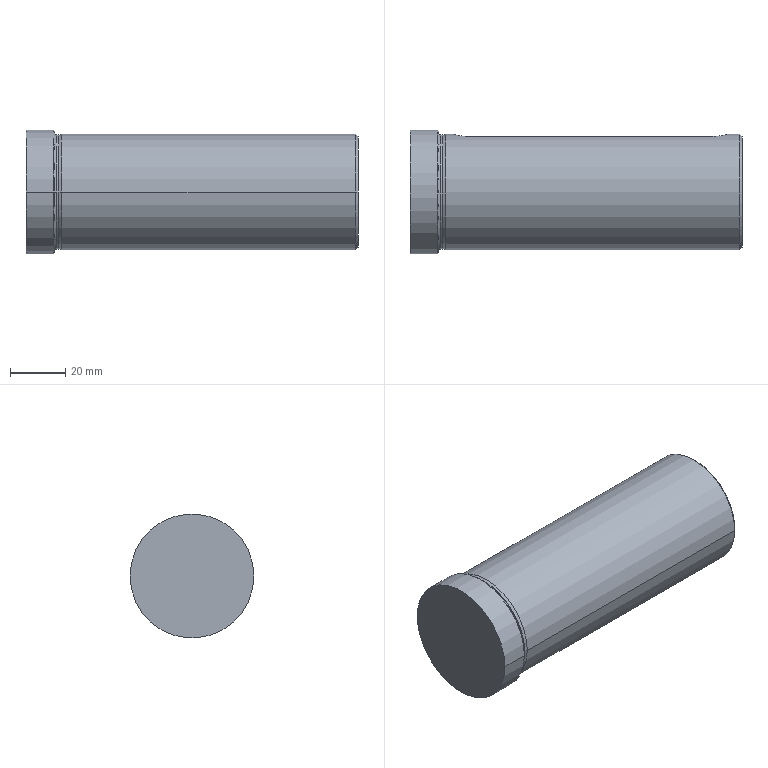Part | STEP file | Input 106 | 1 solid | 35 faces | box 120.5 x 45 x 45 mm | volume 154941 mm3 | cylinder 13 | cone 10 | torus 6 | plane 6 | commonest cylinder face diameters 12 x3 14 x2 17 x2 41.4 x2 42 x2 45 x2